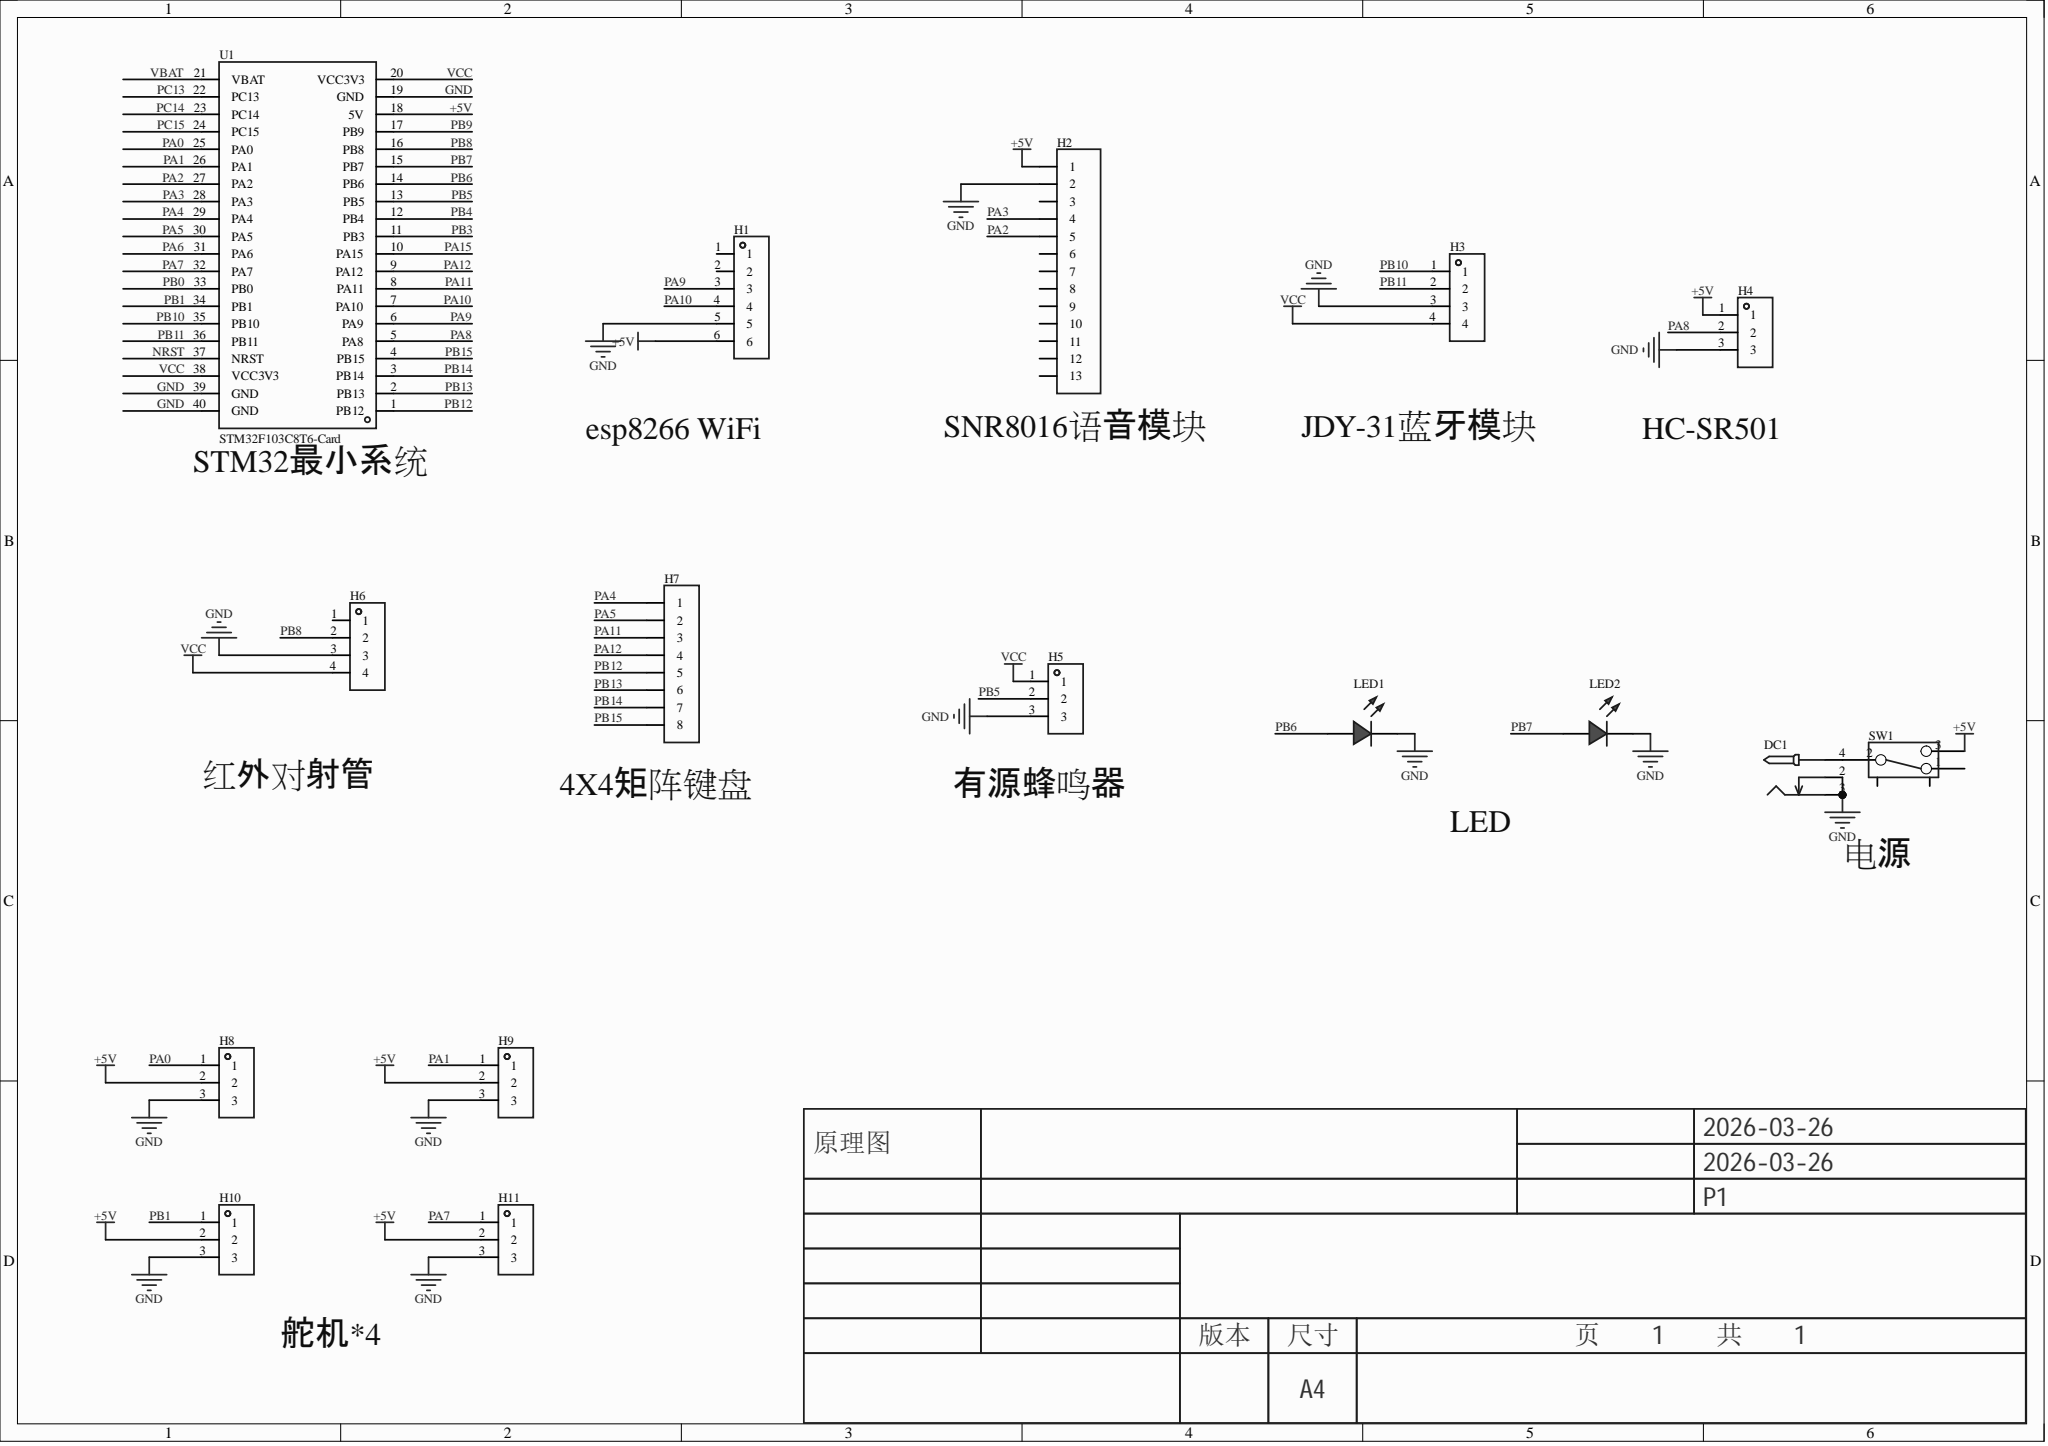Circuit board | Altium Designer | 16 parts | 27 nets
Bill of materials:
Comment,Description,Designator,Footprint,LibRef,Quantity
"","","DC1","DC-2.0","DC-005_2.0","1"
"","","H1","HDR-TH_6P-P2.54-V-F","HDR-F_2.54_1x6P","1"
"","","H2","HDR-TH_13P-P2.54-V-F","HDR-F_2.54_1x13P","1"
"","","H3, H6","HDR-TH_4P-P2.54-V-F","HDR-F_2.54_1x4P","2"
"","","H4, H5, H8, H9, H10, H11","HDR-TH_3P-P2.54-V-F","HDR-F_2.54_1x3P","6"
"","","H7","HDR-TH_8P-P2.54-V-F-1","HDR-F_2.54_1x8P","1"
"","","LED1, LED2","LED-TH_5mm","LED_TH-R_5mm","2"
"","","SW1","拨动开关","拨动开关_正","1"
"STM32F103C8T6-Card","","U1","CONN-TH_L53.3-W22.9_STM32F103C8T6-CARD","STM32F103C8T6-Card","1"
Netlist (Protel format):
[
DC1
DC-2.0




]
[
H1
HDR-TH_6P-P2.54-V-F




]
[
H2
HDR-TH_13P-P2.54-V-F




]
[
H3
HDR-TH_4P-P2.54-V-F




]
[
H4
HDR-TH_3P-P2.54-V-F




]
[
H5
HDR-TH_3P-P2.54-V-F




]
[
H6
HDR-TH_4P-P2.54-V-F




]
[
H7
HDR-TH_8P-P2.54-V-F-1




]
[
H8
HDR-TH_3P-P2.54-V-F




]
[
H9
HDR-TH_3P-P2.54-V-F




]
[
H10
HDR-TH_3P-P2.54-V-F




]
[
H11
HDR-TH_3P-P2.54-V-F




]
[
LED1
LED-TH_5mm




]
[
LED2
LED-TH_5mm




]
[
SW1
拨动开关




]
[
U1
CONN-TH_L53.3-W22.9_STM32F103C8T6-CARD
STM32F103C8T6-Card



]
(
VCC
H3-4
H5-1
H6-4
U1-20
U1-38
)
(
PB15
H7-8
U1-4
)
(
PB14
H7-7
U1-3
)
(
PB13
H7-6
U1-2
)
(
PB12
H7-5
U1-1
)
(
PB11
H3-2
U1-36
)
(
PB10
H3-1
U1-35
)
(
PB8
H6-2
U1-16
)
(
PB7
LED2-1
U1-15
)
(
PB6
LED1-1
U1-14
)
(
PB5
H5-2
U1-13
)
(
PB1
H10-1
U1-34
)
(
PA12
H7-4
U1-9
)
(
PA11
H7-3
U1-8
)
(
PA10
H1-4
U1-7
)
(
PA9
H1-3
U1-6
)
(
PA8
H4-2
U1-5
)
(
PA7
H11-1
U1-32
)
(
PA5
H7-2
U1-30
)
(
PA4
H7-1
U1-29
)
(
PA3
H2-4
U1-28
)
(
PA2
H2-5
U1-27
)
(
PA1
H9-1
U1-26
)
(
PA0
H8-1
U1-25
)
(
NetDC1_4
DC1-4
SW1-2
)
(
GND
DC1-2
DC1-3
H1-5
H2-2
H3-3
H4-3
H5-3
H6-3
H8-3
H9-3
H10-3
H11-3
LED1-2
LED2-2
U1-19
U1-39
U1-40
)
(
+5V
H1-6
H2-1
H4-1
H8-2
H9-2
H10-2
H11-2
SW1-3
U1-18
)